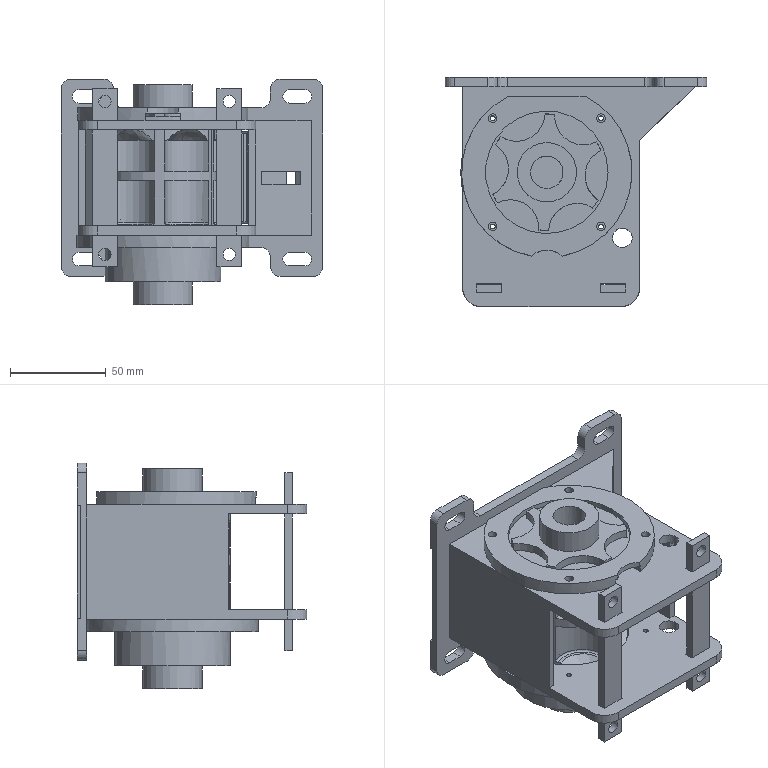Part | NX | features EXTRUDE 14, DATUM_CSYS 8, SKETCH 8, BREP 4, LINKED_FACE 4, EXTRACT_BODY 3, EXTRACT_DATUM_PLANE 3, UNITE 3, INTERSECT 1, Pattern Geometry 1, REPLACE_FACE 1 | 12 solids | 449 faces | box 136.5 x 120 x 117.9 mm | volume 352197 mm3 | plane 244 | cylinder 155 | sphere 30 | cone 14 | torus 6 | commonest cylinder face diameters 30 x32 2.5 x16 17 x14 61 x13 10 x12 54 x12